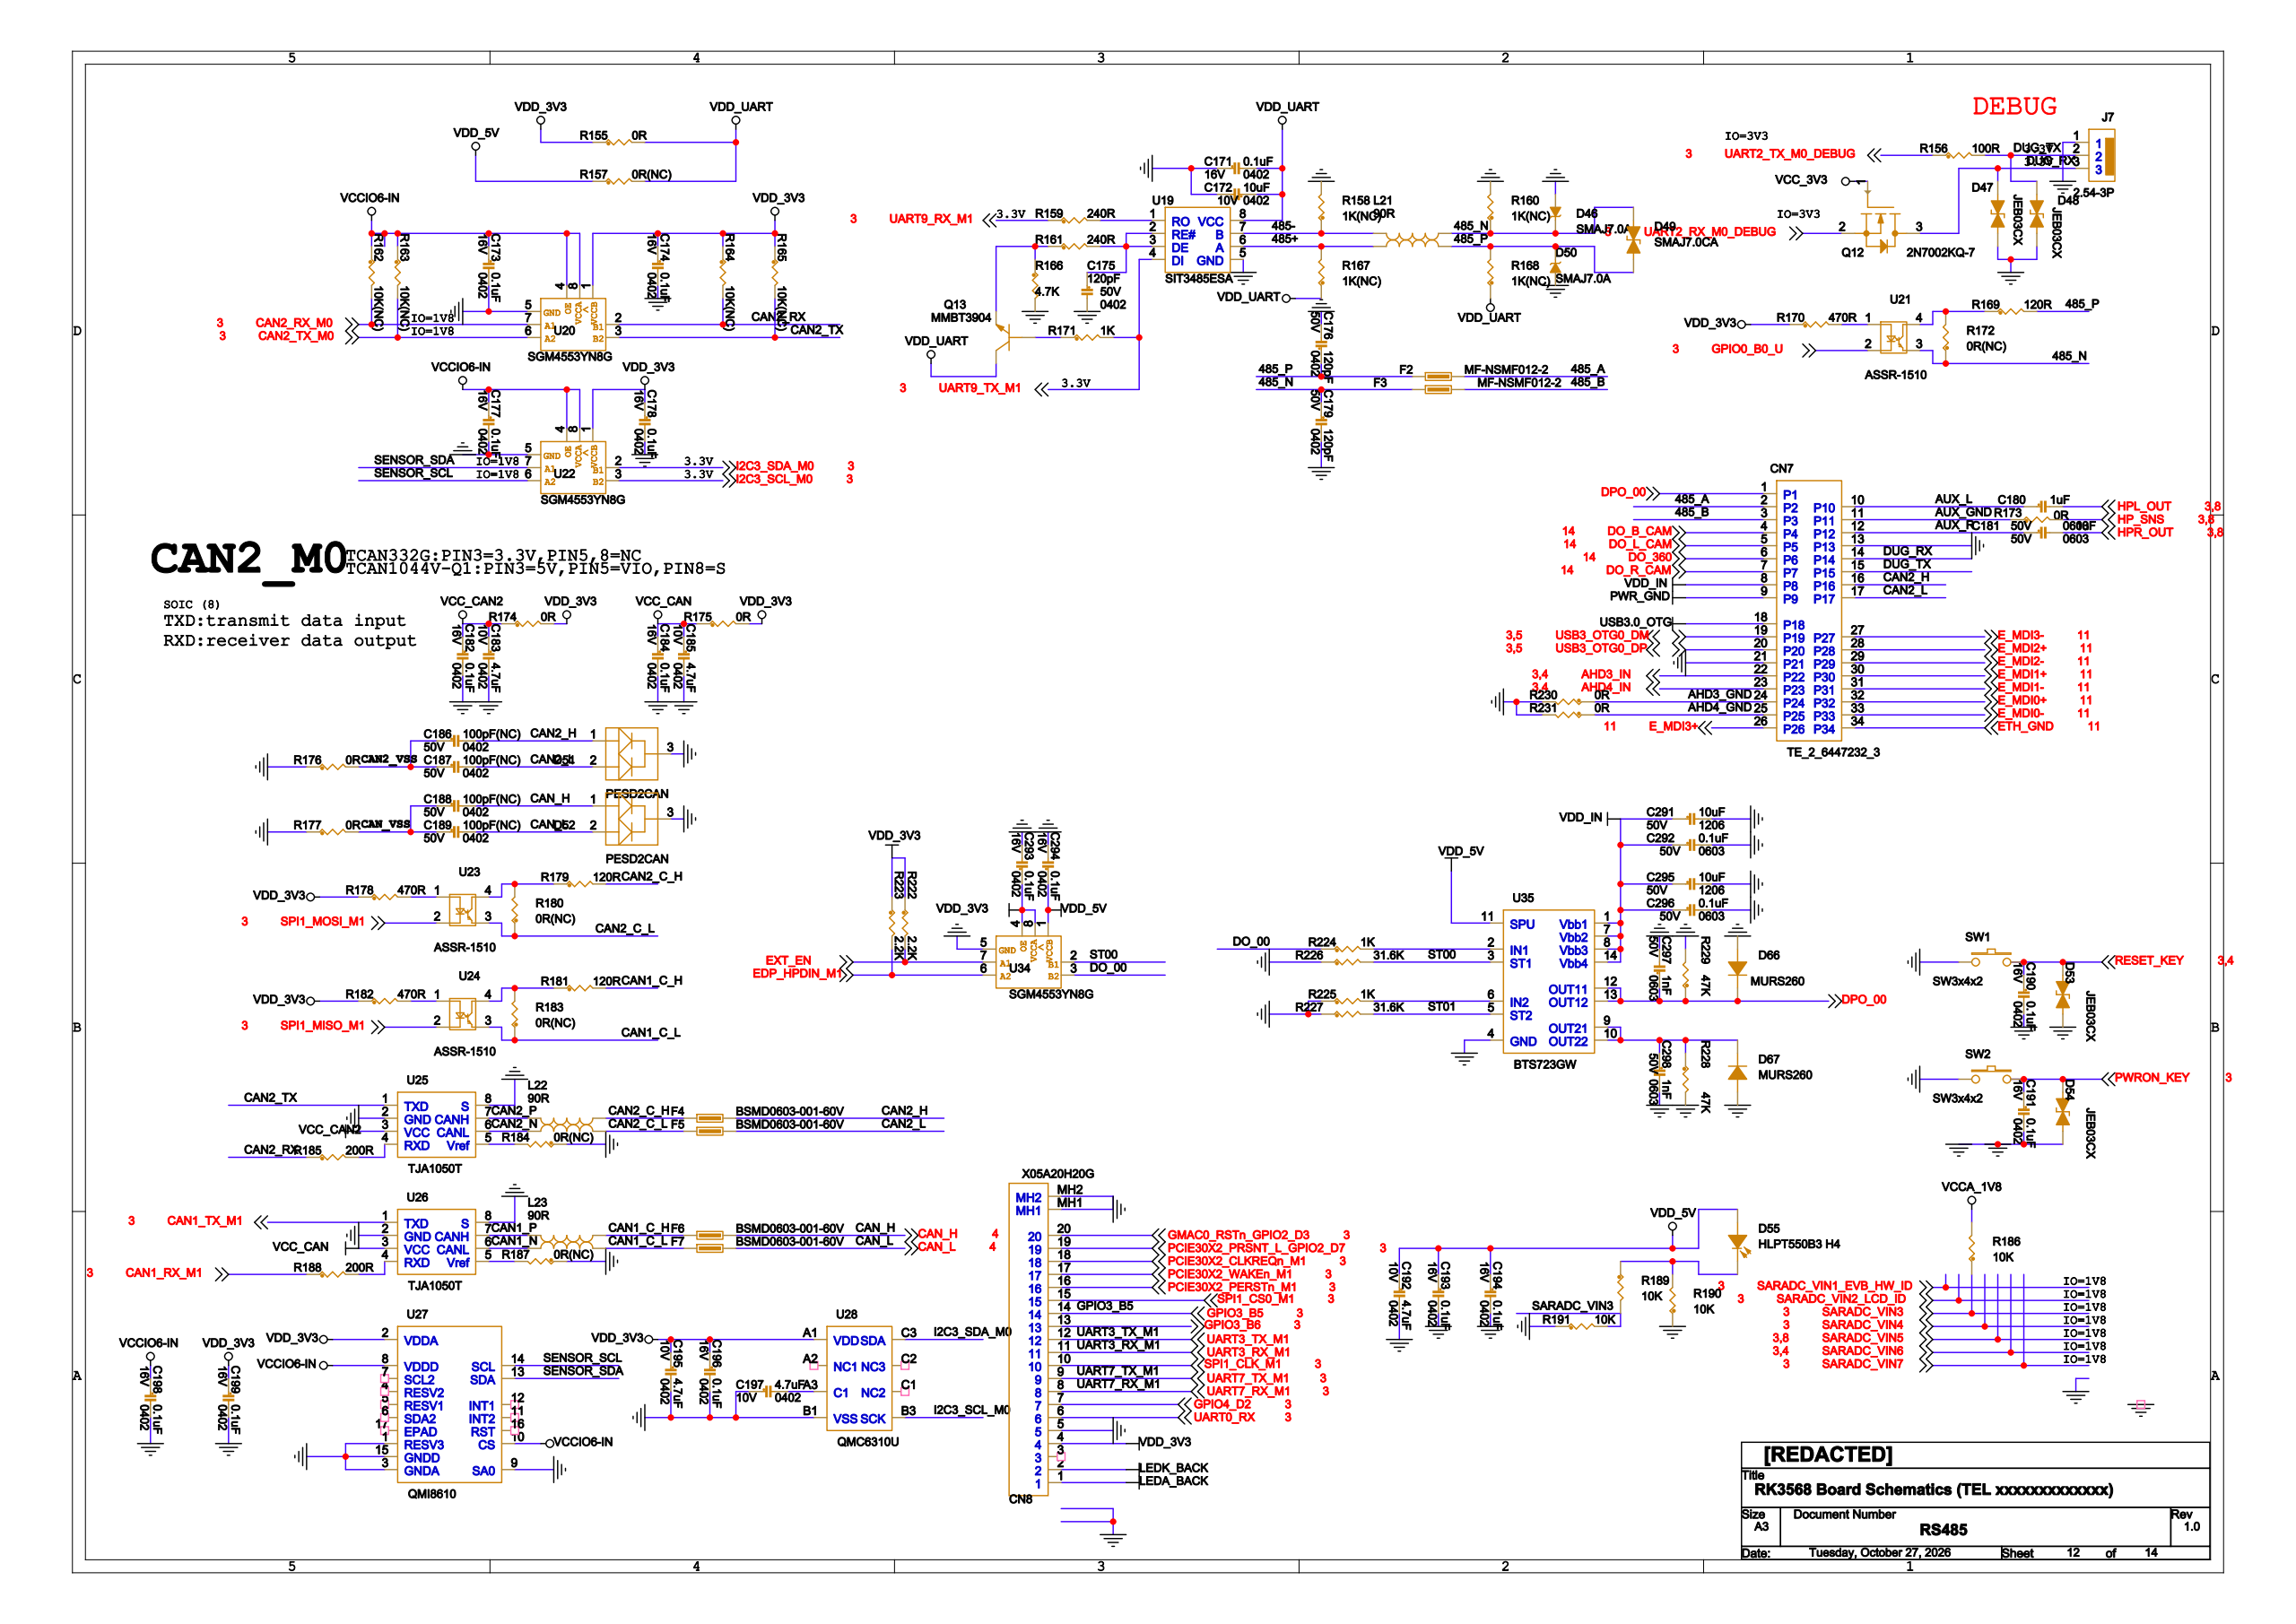Circuit board | Cadence Allegro | 669 parts | 581 nets | one sheet of the schematic
Parts on this sheet (reference | value | footprint):
C171 | 0.1uF | C0402
C172 | 10uF | C0402
C173 | 0.1uF | C0402
C174 | 0.1uF | C0402
C175 | 120pF | C0402
C176 | 120pF | C0402
C177 | 0.1uF | C0402
C178 | 0.1uF | C0402
C179 | 120pF | C0402
C180 | 1uF | C0603
C181 | 1uF | C0603
C182 | 0.1uF | C0402
C183 | 4.7uF | C0402
C184 | 0.1uF | C0402
C185 | 4.7uF | C0402
C186 | 100pF(NC) | C0402
C187 | 100pF(NC) | C0402
C188 | 100pF(NC) | C0402
C189 | 100pF(NC) | C0402
C190 | 0.1uF | C0402
C191 | 0.1uF | C0402
C192 | 4.7uF | C0402
C193 | 0.1uF | C0402
C194 | 0.1uF | C0402
C195 | 4.7uF | C0402
C196 | 0.1uF | C0402
C197 | 4.7uF | C0402
C198 | 0.1uF | C0402
C199 | 0.1uF | C0402
C291 | 10uF | C1206
C292 | 0.1uF | C0603
C293 | 0.1uF | C0402
C294 | 0.1uF | C0402
C295 | 10uF | C1206
C296 | 0.1uF | C0603
C297 | 1nF | C0603
C298 | 1nF | C0603
CN7 | TE_2_6447232_3 | TE_2-6447232-3
CN8 | X05A20H20G | FPC-20-0P5-2MMH
D46 | SMAJ7.0A | SMA
D47 | JEB03CX | SOD323
D48 | JEB03CX | SOD323
D49 | SMAJ7.0CA | SMA
D50 | SMAJ7.0A | SMA
D51 | PESD2CAN | SOT-23
D52 | PESD2CAN | SOT-23
D53 | JEB03CX | SOD323
D54 | JEB03CX | SOD323
D55 | HLPT550B3 H4 | LED_D3MM
D66 | MURS260 | SMA
D67 | MURS260 | SMA
F2 | MF-NSMF012-2 | R1206
F3 | MF-NSMF012-2 | R1206
F4 | BSMD0603-001-60V | R0603
F5 | BSMD0603-001-60V | R0603
F6 | BSMD0603-001-60V | R0603
F7 | BSMD0603-001-60V | R0603
J7 | 2.54-3P | SIP2P54_3
L21 | 90R | WCM2012
L22 | 90R | WCM2012
L23 | 90R | WCM2012
Q12 | 2N7002KQ-7 | SOT-23
Q13 | MMBT3904 | SOT-23
R155 | 0R | R0402
R156 | 100R | R0402
R157 | 0R(NC) | R0402
R158 | 1K(NC) | R0402
R159 | 240R | R0402
R160 | 1K(NC) | R0402
R161 | 240R | R0402
R162 | 10K(NC) | R0402
R163 | 10K(NC) | R0402
R164 | 10K(NC) | R0402
R165 | 10K(NC) | R0402
R166 | 4.7K | R0402
R167 | 1K(NC) | R0402
R168 | 1K(NC) | R0402
R169 | 120R | R0805
R170 | 470R | R0402
R171 | 1K | R0402
R172 | 0R(NC) | R0603
R173 | 0R | R0402
R174 | 0R | R0402
R175 | 0R | R0402
R176 | 0R | R0402
R177 | 0R | R0402
R178 | 470R | R0402
R179 | 120R | R0805
R180 | 0R(NC) | R0603
R181 | 120R | R0805
R182 | 470R | R0402
R183 | 0R(NC) | R0603
R184 | 0R(NC) | R0402
R185 | 200R | R0402
R186 | 10K | R0402
R187 | 0R(NC) | R0402
R188 | 200R | R0402
R189 | 10K | R0402
R190 | 10K | R0402
R191 | 10K | R0402
R222 | 2.2K | R0402
R223 | 2.2K | R0402
R224 | 1K | R0402
R225 | 1K | R0402
R226 | 31.6K | R0402
R227 | 31.6K | R0402
R228 | 47K | R0805
R229 | 47K | R0805
R230 | 0R | R0402
R231 | 0R | R0402
SW1 | SW3x4x2 | SW3X4X2
SW2 | SW3x4x2 | SW3X4X2
U19 | SIT3485ESA | SO8
U20 | SGM4553YN8G | SOT23_8
U21 | ASSR-1510 | SO4
U22 | SGM4553YN8G | SOT23_8
U23 | ASSR-1510 | SO4
U24 | ASSR-1510 | SO4
U25 | TJA1050T | SO8
U26 | TJA1050T | SO8
U27 | QMI8610 | LGA16
U28 | QMC6310U | LGA8
U34 | SGM4553YN8G | SOT23_8
U35 | BTS723GW | SO14
Nets of these parts (net: part-pin ...):
PWR_GND: C291-2 C292-2 C295-2 C296-2 C297-2 C298-2 D66-1 D67-1 R228-2 R229-2 CN7-9
DPO_00: C297-1 D66-2 R229-1 U35-12 U35-13 CN7-1
N84785452: C298-1 D67-2 R228-1 U35-9 U35-10
GND: C171-1 C172-2 C173-2 C174-2 C175-2 C176-2 C177-2 C178-2 C179-2 C182-2 C183-2 C184-2 C185-2 C190-2 C191-2 C192-2 C193-2 C194-2 C195-2 C196-2 C197-1 C198-2 C199-2 C293-2 C294-2 D46-1 D47-1 D48-1 D50-1 D51-3 D52-3 D53-2 D54-2 J7-1 R158-2 R160-2 R166-2 R176-1 R177-1 R184-1 R187-1 R190-1 R191-1 R225-1 R226-1 R227-1 R230-2 R231-2 SW1-1 SW2-1 U19-5 U20-5 U22-5 U25-2 U25-8 U26-2 U26-8 U27-1 U27-3 U27-9 U27-15 U28-B1 U34-5 U35-4 CN7-13 CN7-21 CN8-5 CN8-MH1 CN8-MH2
N84785301: R224-2 U35-2
N84785306: R225-2 U35-6
VDD_5V: C192-1 C193-1 C194-1 C294-1 D55-1 R157-1 U34-1 U35-11
ST00: R226-2 U34-2 U35-3
ST01: R227-2 U35-5
VDD_IN: C291-1 C292-1 C295-1 C296-1 U35-1 U35-7 U35-8 U35-14 CN7-8
VCC3V3_SYS: C174-1 C178-1 C195-1 C196-1 C199-1 C293-1 R155-1 R164-1 R165-1 R170-1 R174-2 R175-2 R178-1 R182-1 R222-1 R223-1 U20-1 U22-1 U27-2 U28-A1 U34-4 U34-8 CN8-4
DUG_TX: D48-2 J7-2 R156-2 CN7-15
DUG_RX: D47-2 J7-3 Q12-3 CN7-14
LEDA_BACK: CN8-1
VCCIO6-IN: C173-1 C177-1 C198-1 R162-1 R163-1 U20-4 U20-8 U22-4 U22-8 U27-8 U27-10
HPR_OUT: C181-2
AUX_L: C180-1 CN7-10
HPL_OUT: C180-2
AUX_R: C181-1 CN7-12
VDD_UART: C171-2 C172-1 Q13-3 R155-2 R157-2 R167-1 R168-1 U19-8
VCC_CAN2: C182-1 C183-1 R174-1 U25-3
VCC_CAN: C184-1 C185-1 R175-1 U26-3
RESET_KEY: C190-1 D53-1 SW1-2
PWRON_KEY: C191-1 D54-1 SW2-2
USB3.0_OTG: CN7-18
N84328482: C197-2 U28-A3
AHD3_IN: CN7-22
AHD4_IN: CN7-23
N84296985: C175-1 R161-2 U19-2 U19-3
485_P: C176-1 D49-1 D50-2 F2-1 L21-4 R168-2 R169-2
485_N: C179-1 D46-2 D49-2 F3-1 L21-2 R160-1 R172-1 U21-3
CAN2_VSS: C186-1 C187-1 R176-2
CAN2_H: C186-2 D51-1 F4-2 CN7-16
CAN_VSS: C188-1 C189-1 R177-2
CAN_L: C189-2 D52-2 F7-2
CAN2_L: C187-2 D51-2 F5-2 CN7-17
CAN_H: C188-2 D52-1 F6-2
E_MDI1+: CN7-30
E_MDI1-: CN7-31
E_MDI0+: CN7-32
E_MDI0-: CN7-33
SPI1_CLK_M1: CN8-10
UART3_RX_M1: CN8-11
UART3_TX_M1: CN8-12
GPIO3_B6: CN8-13
GPIO3_B5: CN8-14
SPI1_CS0_M1: CN8-15
PCIE30X2_PRSNT_L_GPIO2_D7: CN8-19
LEDK_BACK: CN8-2
UART0_RX: CN8-6
GPIO4_D2: CN8-7
UART7_RX_M1: CN8-8
UART7_TX_M1: CN8-9
USB3_OTG0_DP: CN7-20
USB3_OTG0_DM: CN7-19
N84330778: D55-2 R189-1 R190-2
485_A: F2-2 CN7-2
485_B: F3-2 CN7-3
DO_B_CAM: CN7-4
DO_R_CAM: CN7-7
DO_L_CAM: CN7-5
DO_360: CN7-6
CAN2_C_H: F4-1 L22-2 R179-2
CAN2_C_L: F5-1 L22-4 R180-1 U23-3
CAN1_C_H: F6-1 L23-2 R181-2
CAN1_C_L: F7-1 L23-4 R183-1 U24-3
485-: L21-1 R158-1 U19-7
485+: L21-3 R167-2 U19-6
CAN2_P: L22-1 U25-7
CAN2_N: L22-3 U25-6
CAN1_P: L23-1 U26-7
CAN1_N: L23-3 U26-6
VCC_3V3: Q12-1
UART2_RX_M0_DEBUG: Q12-2
N84667213: R184-2 U25-5
N84668269: R187-2 U26-5
AHD3_GND: R230-1 CN7-24
AHD4_GND: R231-1 CN7-25
ETH_GND: CN7-34
AUX_GND: R173-1 CN7-11
HP_SNS: R173-2
CAN2_RX_M0: R162-2 U20-7
CAN2_TX_M0: R163-2 U20-6
CAN2_RX: R164-2 R185-1 U20-2
CAN2_TX: R165-2 U20-3 U25-1
SARADC_VIN3: R186-1 R189-2 R191-2
VCCA_1V8: R186-2
UART2_TX_M0_DEBUG: R156-1
DO_00: R224-1 U34-3
N84624715: Q13-1 R171-1
UART9_TX_M1: R171-2 U19-4
N84303806: Q13-2 R161-1 R166-1
UART9_RX_M1: R159-1
N84296982: R159-2 U19-1
N84296355: R169-1 R172-2 U21-4
N84669448: R179-1 R180-2 U23-4
N84669800: R181-1 R183-2 U24-4
N84296276: R170-2 U21-1
N84669444: R178-2 U23-1
N84669796: R182-2 U24-1
N84667189: R185-2 U25-4
CAN1_RX_M1: R188-1
N84668257: R188-2 U26-4
EXT_EN: R222-2 U34-7
EDP_HPDIN_M1: R223-2 U34-6
E_MDI3+: CN7-26
E_MDI3-: CN7-27
E_MDI2+: CN7-28
E_MDI2-: CN7-29
GPIO0_B0_U: U21-2
SPI1_MOSI_M1: U23-2
SPI1_MISO_M1: U24-2
I2C3_SCL_M0: U22-3 U28-B3
I2C3_SDA_M0: U22-2 U28-C3
SENSOR_SCL: U22-6 U27-14
SENSOR_SDA: U22-7 U27-13
CAN1_TX_M1: U26-1